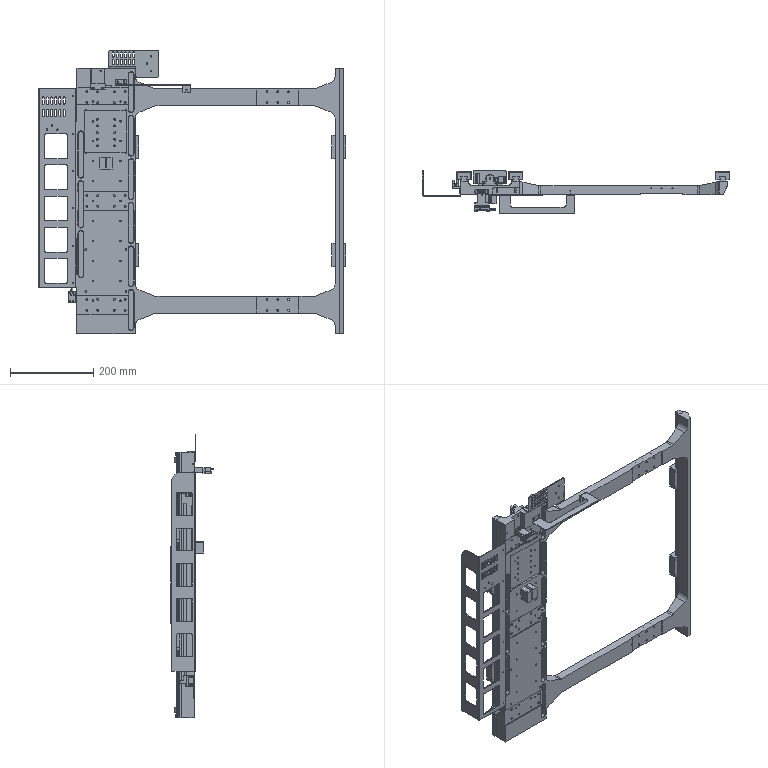Part | NX | features BREP 27 | 38 solids | 3778 faces | volume 4255848 mm3 | plane 2078 | cylinder 1165 | cone 441 | spline 82 | torus 12 | commonest cylinder face diameters 3.3 x212 4.5 x210 10 x119 5 x76 7.5 x66 2.5 x64